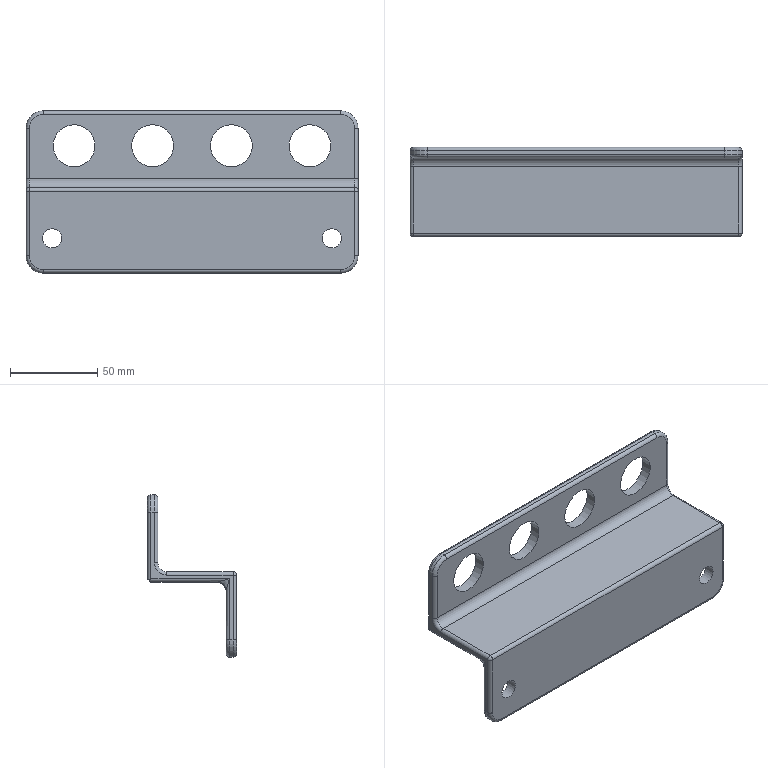Part | NX | features solid 2 | 1 solid | 54 faces | box 190 x 51 x 93 mm | volume 145209 mm3 | cylinder 29 | plane 11 | torus 10 | sphere 2 | spline 2 | commonest cylinder face diameters 4 x17 20 x4 24 x4 10 x2 11 x2
STEP:
#1=CARTESIAN_POINT('',(810.,-500.,212.));
#2=VERTEX_POINT('',#1);
#3=CARTESIAN_POINT('',(810.,-500.,200.));
#4=DIRECTION('',(0.,-1.,0.));
#5=DIRECTION('',(0.,0.,1.));
#6=AXIS2_PLACEMENT_3D('',#3,#4,#5);
#7=CIRCLE('',#6,12.);
#8=EDGE_CURVE('',#2,#2,#7,.T.);
#9=ORIENTED_EDGE('',*,*,#8,.T.);
#10=EDGE_LOOP('',(#9));
#11=FACE_BOUND('',#10,.T.);
#12=CARTESIAN_POINT('',(855.,-500.,212.));
#13=VERTEX_POINT('',#12);
#14=CARTESIAN_POINT('',(855.,-500.,200.));
#15=DIRECTION('',(0.,1.,0.));
#16=DIRECTION('',(0.,0.,1.));
#17=AXIS2_PLACEMENT_3D('',#14,#15,#16);
#18=CIRCLE('',#17,12.);
#19=EDGE_CURVE('',#13,#13,#18,.T.);
#20=ORIENTED_EDGE('',*,*,#19,.F.);
#21=EDGE_LOOP('',(#20));
#22=FACE_BOUND('',#21,.T.);
#23=CARTESIAN_POINT('',(702.5,-500.,218.));
#24=VERTEX_POINT('',#23);
#25=CARTESIAN_POINT('',(872.5,-500.,218.));
#26=VERTEX_POINT('',#25);
#27=CARTESIAN_POINT('',(877.5,-500.,218.));
#28=DIRECTION('',(-1.,0.,0.));
#29=VECTOR('',#28,1000.);
#30=LINE('',#27,#29);
#31=EDGE_CURVE('',#24,#26,#30,.F.);
#32=ORIENTED_EDGE('',*,*,#31,.T.);
#33=CARTESIAN_POINT('',(880.5,-500.,210.));
#34=VERTEX_POINT('',#33);
#35=CARTESIAN_POINT('',(872.5,-500.,210.));
#36=DIRECTION('',(0.,-1.,0.));
#37=DIRECTION('',(0.,0.,1.));
#38=AXIS2_PLACEMENT_3D('',#35,#36,#37);
#39=CIRCLE('',#38,8.);
#40=EDGE_CURVE('',#26,#34,#39,.F.);
#41=ORIENTED_EDGE('',*,*,#40,.T.);
#42=CARTESIAN_POINT('',(880.5,-500.,172.));
#43=VERTEX_POINT('',#42);
#44=CARTESIAN_POINT('',(880.5,-500.,181.));
#45=DIRECTION('',(0.,0.,1.));
#46=VECTOR('',#45,1000.);
#47=LINE('',#44,#46);
#48=EDGE_CURVE('',#34,#43,#47,.F.);
#49=ORIENTED_EDGE('',*,*,#48,.T.);
#50=CARTESIAN_POINT('',(694.5,-500.,172.));
#51=VERTEX_POINT('',#50);
#52=CARTESIAN_POINT('',(827.5,-500.,172.));
#53=DIRECTION('',(1.,0.,0.));
#54=VECTOR('',#53,1000.);
#55=LINE('',#52,#54);
#56=EDGE_CURVE('',#51,#43,#55,.T.);
#57=ORIENTED_EDGE('',*,*,#56,.F.);
#58=CARTESIAN_POINT('',(694.5,-500.,210.));
#59=VERTEX_POINT('',#58);
#60=CARTESIAN_POINT('',(694.5,-500.,181.));
#61=DIRECTION('',(0.,0.,1.));
#62=VECTOR('',#61,1000.);
#63=LINE('',#60,#62);
#64=EDGE_CURVE('',#59,#51,#63,.F.);
#65=ORIENTED_EDGE('',*,*,#64,.F.);
#66=CARTESIAN_POINT('',(702.5,-500.,210.));
#67=DIRECTION('',(0.,1.,0.));
#68=DIRECTION('',(0.,0.,1.));
#69=AXIS2_PLACEMENT_3D('',#66,#67,#68);
#70=CIRCLE('',#69,8.);
#71=EDGE_CURVE('',#24,#59,#70,.F.);
#72=ORIENTED_EDGE('',*,*,#71,.F.);
#73=EDGE_LOOP('',(#32,#41,#49,#57,#65,#72));
#74=FACE_BOUND('',#73,.T.);
#75=CARTESIAN_POINT('',(765.,-500.,212.));
#76=VERTEX_POINT('',#75);
#77=CARTESIAN_POINT('',(765.,-500.,200.));
#78=DIRECTION('',(0.,1.,0.));
#79=DIRECTION('',(0.,0.,1.));
#80=AXIS2_PLACEMENT_3D('',#77,#78,#79);
#81=CIRCLE('',#80,12.);
#82=EDGE_CURVE('',#76,#76,#81,.T.);
#83=ORIENTED_EDGE('',*,*,#82,.F.);
#84=EDGE_LOOP('',(#83));
#85=FACE_BOUND('',#84,.T.);
#86=CARTESIAN_POINT('',(720.,-500.,212.));
#87=VERTEX_POINT('',#86);
#88=CARTESIAN_POINT('',(720.,-500.,200.));
#89=DIRECTION('',(0.,-1.,0.));
#90=DIRECTION('',(0.,0.,1.));
#91=AXIS2_PLACEMENT_3D('',#88,#89,#90);
#92=CIRCLE('',#91,12.);
#93=EDGE_CURVE('',#87,#87,#92,.T.);
#94=ORIENTED_EDGE('',*,*,#93,.T.);
#95=EDGE_LOOP('',(#94));
#96=FACE_BOUND('',#95,.T.);
#97=CARTESIAN_POINT('',(767.5,-500.,170.));
#98=DIRECTION('',(0.,-1.,0.));
#99=DIRECTION('',(0.,0.,1.));
#100=AXIS2_PLACEMENT_3D('',#97,#98,#99);
#101=PLANE('',#100);
#102=ADVANCED_FACE('',(#11,#22,#74,#85,#96),#101,.F.);
#103=CARTESIAN_POINT('',(855.,-506.,212.));
#104=VERTEX_POINT('',#103);
#105=CARTESIAN_POINT('',(855.,-506.,200.));
#106=DIRECTION('',(0.,1.,0.));
#107=DIRECTION('',(0.,0.,1.));
#108=AXIS2_PLACEMENT_3D('',#105,#106,#107);
#109=CIRCLE('',#108,12.);
#110=EDGE_CURVE('',#104,#104,#109,.T.);
#111=ORIENTED_EDGE('',*,*,#110,.T.);
#112=EDGE_LOOP('',(#111));
#113=FACE_BOUND('',#112,.T.);
#114=CARTESIAN_POINT('',(810.,-506.,212.));
#115=VERTEX_POINT('',#114);
#116=CARTESIAN_POINT('',(810.,-506.,200.));
#117=DIRECTION('',(0.,-1.,0.));
#118=DIRECTION('',(0.,0.,1.));
#119=AXIS2_PLACEMENT_3D('',#116,#117,#118);
#120=CIRCLE('',#119,12.);
#121=EDGE_CURVE('',#115,#115,#120,.T.);
#122=ORIENTED_EDGE('',*,*,#121,.F.);
#123=EDGE_LOOP('',(#122));
#124=FACE_BOUND('',#123,.T.);
#125=CARTESIAN_POINT('',(694.5,-506.,181.));
#126=VERTEX_POINT('',#125);
#127=CARTESIAN_POINT('',(880.5,-506.,181.));
#128=VERTEX_POINT('',#127);
#129=CARTESIAN_POINT('',(827.5,-506.,181.));
#130=DIRECTION('',(1.,0.,0.));
#131=VECTOR('',#130,1000.);
#132=LINE('',#129,#131);
#133=EDGE_CURVE('',#126,#128,#132,.T.);
#134=ORIENTED_EDGE('',*,*,#133,.T.);
#135=CARTESIAN_POINT('',(880.5,-506.,210.));
#136=VERTEX_POINT('',#135);
#137=CARTESIAN_POINT('',(880.5,-506.,170.));
#138=DIRECTION('',(0.,0.,1.));
#139=VECTOR('',#138,1000.);
#140=LINE('',#137,#139);
#141=EDGE_CURVE('',#128,#136,#140,.T.);
#142=ORIENTED_EDGE('',*,*,#141,.T.);
#143=CARTESIAN_POINT('',(872.5,-506.,218.));
#144=VERTEX_POINT('',#143);
#145=CARTESIAN_POINT('',(872.5,-506.,210.));
#146=DIRECTION('',(0.,-1.,0.));
#147=DIRECTION('',(0.,0.,1.));
#148=AXIS2_PLACEMENT_3D('',#145,#146,#147);
#149=CIRCLE('',#148,8.);
#150=EDGE_CURVE('',#136,#144,#149,.T.);
#151=ORIENTED_EDGE('',*,*,#150,.T.);
#152=CARTESIAN_POINT('',(702.5,-506.,218.));
#153=VERTEX_POINT('',#152);
#154=CARTESIAN_POINT('',(827.5,-506.,218.));
#155=DIRECTION('',(-1.,0.,0.));
#156=VECTOR('',#155,1000.);
#157=LINE('',#154,#156);
#158=EDGE_CURVE('',#144,#153,#157,.T.);
#159=ORIENTED_EDGE('',*,*,#158,.T.);
#160=CARTESIAN_POINT('',(694.5,-506.,210.));
#161=VERTEX_POINT('',#160);
#162=CARTESIAN_POINT('',(702.5,-506.,210.));
#163=DIRECTION('',(0.,1.,0.));
#164=DIRECTION('',(0.,0.,1.));
#165=AXIS2_PLACEMENT_3D('',#162,#163,#164);
#166=CIRCLE('',#165,8.);
#167=EDGE_CURVE('',#161,#153,#166,.T.);
#168=ORIENTED_EDGE('',*,*,#167,.F.);
#169=CARTESIAN_POINT('',(694.5,-506.,170.));
#170=DIRECTION('',(0.,0.,1.));
#171=VECTOR('',#170,1000.);
#172=LINE('',#169,#171);
#173=EDGE_CURVE('',#126,#161,#172,.T.);
#174=ORIENTED_EDGE('',*,*,#173,.F.);
#175=EDGE_LOOP('',(#134,#142,#151,#159,#168,#174));
#176=FACE_BOUND('',#175,.T.);
#177=CARTESIAN_POINT('',(720.,-506.,212.));
#178=VERTEX_POINT('',#177);
#179=CARTESIAN_POINT('',(720.,-506.,200.));
#180=DIRECTION('',(0.,-1.,0.));
#181=DIRECTION('',(0.,0.,1.));
#182=AXIS2_PLACEMENT_3D('',#179,#180,#181);
#183=CIRCLE('',#182,12.);
#184=EDGE_CURVE('',#178,#178,#183,.T.);
#185=ORIENTED_EDGE('',*,*,#184,.F.);
#186=EDGE_LOOP('',(#185));
#187=FACE_BOUND('',#186,.T.);
#188=CARTESIAN_POINT('',(765.,-506.,212.));
#189=VERTEX_POINT('',#188);
#190=CARTESIAN_POINT('',(765.,-506.,200.));
#191=DIRECTION('',(0.,1.,0.));
#192=DIRECTION('',(0.,0.,1.));
#193=AXIS2_PLACEMENT_3D('',#190,#191,#192);
#194=CIRCLE('',#193,12.);
#195=EDGE_CURVE('',#189,#189,#194,.T.);
#196=ORIENTED_EDGE('',*,*,#195,.T.);
#197=EDGE_LOOP('',(#196));
#198=FACE_BOUND('',#197,.T.);
#199=CARTESIAN_POINT('',(827.5,-506.,170.));
#200=DIRECTION('',(0.,-1.,0.));
#201=DIRECTION('',(0.,0.,1.));
#202=AXIS2_PLACEMENT_3D('',#199,#200,#201);
#203=PLANE('',#202);
#204=ADVANCED_FACE('',(#113,#124,#176,#187,#198),#203,.T.);
#205=CARTESIAN_POINT('',(880.5,-502.,170.));
#206=VERTEX_POINT('',#205);
#207=CARTESIAN_POINT('',(694.5,-502.,170.));
#208=VERTEX_POINT('',#207);
#209=CARTESIAN_POINT('',(827.5,-502.,170.));
#210=DIRECTION('',(-1.,0.,0.));
#211=VECTOR('',#210,1000.);
#212=LINE('',#209,#211);
#213=EDGE_CURVE('',#206,#208,#212,.T.);
#214=ORIENTED_EDGE('',*,*,#213,.F.);
#215=CARTESIAN_POINT('',(880.5,-540.,170.));
#216=VERTEX_POINT('',#215);
#217=CARTESIAN_POINT('',(880.5,-530.,170.));
#218=DIRECTION('',(0.,-1.,0.));
#219=VECTOR('',#218,1000.);
#220=LINE('',#217,#219);
#221=EDGE_CURVE('',#216,#206,#220,.F.);
#222=ORIENTED_EDGE('',*,*,#221,.F.);
#223=CARTESIAN_POINT('',(694.5,-540.,170.));
#224=VERTEX_POINT('',#223);
#225=CARTESIAN_POINT('',(769.5,-540.,170.));
#226=DIRECTION('',(1.,0.,0.));
#227=VECTOR('',#226,1000.);
#228=LINE('',#225,#227);
#229=EDGE_CURVE('',#216,#224,#228,.F.);
#230=ORIENTED_EDGE('',*,*,#229,.T.);
#231=CARTESIAN_POINT('',(694.5,-530.,170.));
#232=DIRECTION('',(0.,-1.,0.));
#233=VECTOR('',#232,1000.);
#234=LINE('',#231,#233);
#235=EDGE_CURVE('',#224,#208,#234,.F.);
#236=ORIENTED_EDGE('',*,*,#235,.T.);
#237=EDGE_LOOP('',(#214,#222,#230,#236));
#238=FACE_BOUND('',#237,.T.);
#239=CARTESIAN_POINT('',(827.5,-530.,170.));
#240=DIRECTION('',(0.,0.,-1.));
#241=DIRECTION('',(1.,0.,0.));
#242=AXIS2_PLACEMENT_3D('',#239,#240,#241);
#243=PLANE('',#242);
#244=ADVANCED_FACE('',(#238),#243,.T.);
#245=CARTESIAN_POINT('',(694.5,-511.,176.));
#246=VERTEX_POINT('',#245);
#247=CARTESIAN_POINT('',(880.5,-511.,176.));
#248=VERTEX_POINT('',#247);
#249=CARTESIAN_POINT('',(827.5,-511.,176.));
#250=DIRECTION('',(1.,0.,0.));
#251=VECTOR('',#250,1000.);
#252=LINE('',#249,#251);
#253=EDGE_CURVE('',#246,#248,#252,.T.);
#254=ORIENTED_EDGE('',*,*,#253,.T.);
#255=CARTESIAN_POINT('',(880.5,-511.,181.));
#256=DIRECTION('',(-1.,0.,0.));
#257=DIRECTION('',(0.,0.,1.));
#258=AXIS2_PLACEMENT_3D('',#255,#256,#257);
#259=CIRCLE('',#258,5.);
#260=EDGE_CURVE('',#128,#248,#259,.T.);
#261=ORIENTED_EDGE('',*,*,#260,.F.);
#262=ORIENTED_EDGE('',*,*,#133,.F.);
#263=CARTESIAN_POINT('',(694.5,-511.,181.));
#264=DIRECTION('',(-1.,0.,0.));
#265=DIRECTION('',(0.,0.,1.));
#266=AXIS2_PLACEMENT_3D('',#263,#264,#265);
#267=CIRCLE('',#266,5.);
#268=EDGE_CURVE('',#126,#246,#267,.T.);
#269=ORIENTED_EDGE('',*,*,#268,.T.);
#270=EDGE_LOOP('',(#254,#261,#262,#269));
#271=FACE_BOUND('',#270,.T.);
#272=CARTESIAN_POINT('',(827.5,-511.,181.));
#273=DIRECTION('',(1.,0.,0.));
#274=DIRECTION('',(0.,0.,1.));
#275=AXIS2_PLACEMENT_3D('',#272,#273,#274);
#276=CYLINDRICAL_SURFACE('',#275,5.);
#277=ADVANCED_FACE('',(#271),#276,.F.);
#278=ORIENTED_EDGE('',*,*,#56,.T.);
#279=CARTESIAN_POINT('',(882.232,-501.,171.));
#280=VERTEX_POINT('',#279);
#281=CARTESIAN_POINT('',(880.5,-502.,170.));
#282=DIRECTION('',(0.,0.7071,-0.7071));
#283=DIRECTION('',(0.,0.7071,0.7071));
#284=AXIS2_PLACEMENT_3D('',#281,#282,#283);
#285=ELLIPSE('',#284,2.828,2.);
#286=EDGE_CURVE('',#43,#280,#285,.T.);
#287=ORIENTED_EDGE('',*,*,#286,.T.);
#288=CARTESIAN_POINT('',(880.5,-500.,172.));
#289=DIRECTION('',(0.,0.7071,-0.7071));
#290=DIRECTION('',(0.,-0.7071,-0.7071));
#291=AXIS2_PLACEMENT_3D('',#288,#289,#290);
#292=ELLIPSE('',#291,2.828,2.);
#293=EDGE_CURVE('',#280,#206,#292,.T.);
#294=ORIENTED_EDGE('',*,*,#293,.T.);
#295=ORIENTED_EDGE('',*,*,#213,.T.);
#296=CARTESIAN_POINT('',(692.768,-501.,171.));
#297=VERTEX_POINT('',#296);
#298=CARTESIAN_POINT('',(694.5,-500.,172.));
#299=DIRECTION('',(0.,-0.7071,0.7071));
#300=DIRECTION('',(0.,-0.7071,-0.7071));
#301=AXIS2_PLACEMENT_3D('',#298,#299,#300);
#302=ELLIPSE('',#301,2.828,2.);
#303=EDGE_CURVE('',#297,#208,#302,.T.);
#304=ORIENTED_EDGE('',*,*,#303,.F.);
#305=CARTESIAN_POINT('',(694.5,-502.,170.));
#306=DIRECTION('',(0.,-0.7071,0.7071));
#307=DIRECTION('',(0.,0.7071,0.7071));
#308=AXIS2_PLACEMENT_3D('',#305,#306,#307);
#309=ELLIPSE('',#308,2.828,2.);
#310=EDGE_CURVE('',#51,#297,#309,.T.);
#311=ORIENTED_EDGE('',*,*,#310,.F.);
#312=EDGE_LOOP('',(#278,#287,#294,#295,#304,#311));
#313=FACE_BOUND('',#312,.T.);
#314=CARTESIAN_POINT('',(827.5,-500.,172.));
#315=DIRECTION('',(0.,-0.7071,0.7071));
#316=DIRECTION('',(0.,-0.7071,-0.7071));
#317=AXIS2_PLACEMENT_3D('',#314,#315,#316);
#318=PLANE('',#317);
#319=ADVANCED_FACE('',(#313),#318,.F.);
#320=CARTESIAN_POINT('',(694.5,-549.,176.));
#321=VERTEX_POINT('',#320);
#322=CARTESIAN_POINT('',(880.5,-549.,176.));
#323=VERTEX_POINT('',#322);
#324=CARTESIAN_POINT('',(769.5,-549.,176.));
#325=DIRECTION('',(1.,0.,0.));
#326=VECTOR('',#325,1000.);
#327=LINE('',#324,#326);
#328=EDGE_CURVE('',#321,#323,#327,.T.);
#329=ORIENTED_EDGE('',*,*,#328,.T.);
#330=CARTESIAN_POINT('',(880.5,-551.,176.));
#331=DIRECTION('',(0.,-1.,0.));
#332=VECTOR('',#331,1000.);
#333=LINE('',#330,#332);
#334=EDGE_CURVE('',#323,#248,#333,.F.);
#335=ORIENTED_EDGE('',*,*,#334,.T.);
#336=ORIENTED_EDGE('',*,*,#253,.F.);
#337=CARTESIAN_POINT('',(694.5,-551.,176.));
#338=DIRECTION('',(0.,-1.,0.));
#339=VECTOR('',#338,1000.);
#340=LINE('',#337,#339);
#341=EDGE_CURVE('',#321,#246,#340,.F.);
#342=ORIENTED_EDGE('',*,*,#341,.F.);
#343=EDGE_LOOP('',(#329,#335,#336,#342));
#344=FACE_BOUND('',#343,.T.);
#345=CARTESIAN_POINT('',(769.5,-551.,176.));
#346=DIRECTION('',(0.,0.,1.));
#347=DIRECTION('',(1.,0.,0.));
#348=AXIS2_PLACEMENT_3D('',#345,#346,#347);
#349=PLANE('',#348);
#350=ADVANCED_FACE('',(#344),#349,.T.);
#351=CARTESIAN_POINT('',(873.,-551.,147.));
#352=VERTEX_POINT('',#351);
#353=CARTESIAN_POINT('',(867.5,-551.,147.));
#354=DIRECTION('',(0.,-1.,0.));
#355=DIRECTION('',(1.,0.,0.));
#356=AXIS2_PLACEMENT_3D('',#353,#354,#355);
#357=CIRCLE('',#356,5.5);
#358=EDGE_CURVE('',#352,#352,#357,.T.);
#359=ORIENTED_EDGE('',*,*,#358,.F.);
#360=EDGE_LOOP('',(#359));
#361=FACE_BOUND('',#360,.T.);
#362=CARTESIAN_POINT('',(872.5,-551.,129.));
#363=VERTEX_POINT('',#362);
#364=CARTESIAN_POINT('',(702.5,-551.,129.));
#365=VERTEX_POINT('',#364);
#366=CARTESIAN_POINT('',(827.5,-551.,129.));
#367=DIRECTION('',(1.,0.,0.));
#368=VECTOR('',#367,1000.);
#369=LINE('',#366,#368);
#370=EDGE_CURVE('',#363,#365,#369,.F.);
#371=ORIENTED_EDGE('',*,*,#370,.F.);
#372=CARTESIAN_POINT('',(880.5,-551.,137.));
#373=VERTEX_POINT('',#372);
#374=CARTESIAN_POINT('',(872.5,-551.,137.));
#375=DIRECTION('',(0.,1.,0.));
#376=DIRECTION('',(-1.,0.,0.));
#377=AXIS2_PLACEMENT_3D('',#374,#375,#376);
#378=CIRCLE('',#377,8.);
#379=EDGE_CURVE('',#373,#363,#378,.T.);
#380=ORIENTED_EDGE('',*,*,#379,.F.);
#381=CARTESIAN_POINT('',(880.5,-551.,174.));
#382=VERTEX_POINT('',#381);
#383=CARTESIAN_POINT('',(880.5,-551.,176.));
#384=DIRECTION('',(0.,0.,1.));
#385=VECTOR('',#384,1000.);
#386=LINE('',#383,#385);
#387=EDGE_CURVE('',#373,#382,#386,.T.);
#388=ORIENTED_EDGE('',*,*,#387,.T.);
#389=CARTESIAN_POINT('',(694.5,-551.,174.));
#390=VERTEX_POINT('',#389);
#391=CARTESIAN_POINT('',(769.5,-551.,174.));
#392=DIRECTION('',(-1.,0.,0.));
#393=VECTOR('',#392,1000.);
#394=LINE('',#391,#393);
#395=EDGE_CURVE('',#382,#390,#394,.T.);
#396=ORIENTED_EDGE('',*,*,#395,.T.);
#397=CARTESIAN_POINT('',(694.5,-551.,137.));
#398=VERTEX_POINT('',#397);
#399=CARTESIAN_POINT('',(694.5,-551.,176.));
#400=DIRECTION('',(0.,0.,1.));
#401=VECTOR('',#400,1000.);
#402=LINE('',#399,#401);
#403=EDGE_CURVE('',#398,#390,#402,.T.);
#404=ORIENTED_EDGE('',*,*,#403,.F.);
#405=CARTESIAN_POINT('',(702.5,-551.,137.));
#406=DIRECTION('',(0.,-1.,0.));
#407=DIRECTION('',(1.,0.,0.));
#408=AXIS2_PLACEMENT_3D('',#405,#406,#407);
#409=CIRCLE('',#408,8.);
#410=EDGE_CURVE('',#398,#365,#409,.T.);
#411=ORIENTED_EDGE('',*,*,#410,.T.);
#412=EDGE_LOOP('',(#371,#380,#388,#396,#404,#411));
#413=FACE_BOUND('',#412,.T.);
#414=CARTESIAN_POINT('',(702.,-551.,147.));
#415=VERTEX_POINT('',#414);
#416=CARTESIAN_POINT('',(707.5,-551.,147.));
#417=DIRECTION('',(0.,1.,0.));
#418=DIRECTION('',(-1.,0.,0.));
#419=AXIS2_PLACEMENT_3D('',#416,#417,#418);
#420=CIRCLE('',#419,5.5);
#421=EDGE_CURVE('',#415,#415,#420,.T.);
#422=ORIENTED_EDGE('',*,*,#421,.T.);
#423=EDGE_LOOP('',(#422));
#424=FACE_BOUND('',#423,.T.);
#425=CARTESIAN_POINT('',(769.5,-551.,176.));
#426=DIRECTION('',(0.,1.,0.));
#427=DIRECTION('',(0.,0.,-1.));
#428=AXIS2_PLACEMENT_3D('',#425,#426,#427);
#429=PLANE('',#428);
#430=ADVANCED_FACE('',(#361,#413,#424),#429,.F.);
#431=ORIENTED_EDGE('',*,*,#395,.F.);
#432=CARTESIAN_POINT('',(880.5,-549.,174.));
#433=DIRECTION('',(-1.,0.,0.));
#434=DIRECTION('',(0.,1.,0.));
#435=AXIS2_PLACEMENT_3D('',#432,#433,#434);
#436=CIRCLE('',#435,2.);
#437=EDGE_CURVE('',#382,#323,#436,.T.);
#438=ORIENTED_EDGE('',*,*,#437,.T.);
#439=ORIENTED_EDGE('',*,*,#328,.F.);
#440=CARTESIAN_POINT('',(694.5,-549.,174.));
#441=DIRECTION('',(-1.,0.,0.));
#442=DIRECTION('',(0.,1.,0.));
#443=AXIS2_PLACEMENT_3D('',#440,#441,#442);
#444=CIRCLE('',#443,2.);
#445=EDGE_CURVE('',#390,#321,#444,.T.);
#446=ORIENTED_EDGE('',*,*,#445,.F.);
#447=EDGE_LOOP('',(#431,#438,#439,#446));
#448=FACE_BOUND('',#447,.T.);
#449=CARTESIAN_POINT('',(769.5,-549.,174.));
#450=DIRECTION('',(-1.,0.,0.));
#451=DIRECTION('',(0.,1.,0.));
#452=AXIS2_PLACEMENT_3D('',#449,#450,#451);
#453=CYLINDRICAL_SURFACE('',#452,2.);
#454=ADVANCED_FACE('',(#448),#453,.T.);
#455=CARTESIAN_POINT('',(873.,-545.,147.));
#456=VERTEX_POINT('',#455);
#457=CARTESIAN_POINT('',(867.5,-545.,147.));
#458=DIRECTION('',(0.,-1.,0.));
#459=DIRECTION('',(1.,0.,0.));
#460=AXIS2_PLACEMENT_3D('',#457,#458,#459);
#461=CIRCLE('',#460,5.5);
#462=EDGE_CURVE('',#456,#456,#461,.T.);
#463=ORIENTED_EDGE('',*,*,#462,.T.);
#464=EDGE_LOOP('',(#463));
#465=FACE_BOUND('',#464,.T.);
#466=CARTESIAN_POINT('',(694.5,-545.,165.));
#467=VERTEX_POINT('',#466);
#468=CARTESIAN_POINT('',(880.5,-545.,165.));
#469=VERTEX_POINT('',#468);
#470=CARTESIAN_POINT('',(885.5,-545.,165.));
#471=DIRECTION('',(1.,0.,0.));
#472=VECTOR('',#471,1000.);
#473=LINE('',#470,#472);
#474=EDGE_CURVE('',#467,#469,#473,.T.);
#475=ORIENTED_EDGE('',*,*,#474,.T.);
#476=CARTESIAN_POINT('',(880.5,-545.,137.));
#477=VERTEX_POINT('',#476);
#478=CARTESIAN_POINT('',(880.5,-545.,157.));
#479=DIRECTION('',(0.,0.,-1.));
#480=VECTOR('',#479,1000.);
#481=LINE('',#478,#480);
#482=EDGE_CURVE('',#477,#469,#481,.F.);
#483=ORIENTED_EDGE('',*,*,#482,.F.);
#484=CARTESIAN_POINT('',(872.5,-545.,129.));
#485=VERTEX_POINT('',#484);
#486=CARTESIAN_POINT('',(872.5,-545.,137.));
#487=DIRECTION('',(0.,-1.,0.));
#488=DIRECTION('',(1.,0.,0.));
#489=AXIS2_PLACEMENT_3D('',#486,#487,#488);
#490=CIRCLE('',#489,8.);
#491=EDGE_CURVE('',#485,#477,#490,.T.);
#492=ORIENTED_EDGE('',*,*,#491,.F.);
#493=CARTESIAN_POINT('',(702.5,-545.,129.));
#494=VERTEX_POINT('',#493);
#495=CARTESIAN_POINT('',(827.5,-545.,129.));
#496=DIRECTION('',(-1.,0.,0.));
#497=VECTOR('',#496,1000.);
#498=LINE('',#495,#497);
#499=EDGE_CURVE('',#494,#485,#498,.F.);
#500=ORIENTED_EDGE('',*,*,#499,.F.);
#501=CARTESIAN_POINT('',(694.5,-545.,137.));
#502=VERTEX_POINT('',#501);
#503=CARTESIAN_POINT('',(702.5,-545.,137.));
#504=DIRECTION('',(0.,1.,0.));
#505=DIRECTION('',(-1.,0.,0.));
#506=AXIS2_PLACEMENT_3D('',#503,#504,#505);
#507=CIRCLE('',#506,8.);
#508=EDGE_CURVE('',#494,#502,#507,.T.);
#509=ORIENTED_EDGE('',*,*,#508,.T.);
#510=CARTESIAN_POINT('',(694.5,-545.,157.));
#511=DIRECTION('',(0.,0.,-1.));
#512=VECTOR('',#511,1000.);
#513=LINE('',#510,#512);
#514=EDGE_CURVE('',#502,#467,#513,.F.);
#515=ORIENTED_EDGE('',*,*,#514,.T.);
#516=EDGE_LOOP('',(#475,#483,#492,#500,#509,#515));
#517=FACE_BOUND('',#516,.T.);
#518=CARTESIAN_POINT('',(702.,-545.,147.));
#519=VERTEX_POINT('',#518);
#520=CARTESIAN_POINT('',(707.5,-545.,147.));
#521=DIRECTION('',(0.,1.,0.));
#522=DIRECTION('',(-1.,0.,0.));
#523=AXIS2_PLACEMENT_3D('',#520,#521,#522);
#524=CIRCLE('',#523,5.5);
#525=EDGE_CURVE('',#519,#519,#524,.T.);
#526=ORIENTED_EDGE('',*,*,#525,.F.);
#527=EDGE_LOOP('',(#526));
#528=FACE_BOUND('',#527,.T.);
#529=CARTESIAN_POINT('',(827.5,-545.,157.));
#530=DIRECTION('',(0.,1.,0.));
#531=DIRECTION('',(1.,0.,0.));
#532=AXIS2_PLACEMENT_3D('',#529,#530,#531);
#533=PLANE('',#532);
#534=ADVANCED_FACE('',(#465,#517,#528),#533,.T.);
#535=ORIENTED_EDGE('',*,*,#229,.F.);
#536=CARTESIAN_POINT('',(880.5,-540.,165.));
#537=DIRECTION('',(1.,0.,0.));
#538=DIRECTION('',(0.,-1.,0.));
#539=AXIS2_PLACEMENT_3D('',#536,#537,#538);
#540=CIRCLE('',#539,5.);
#541=EDGE_CURVE('',#216,#469,#540,.T.);
#542=ORIENTED_EDGE('',*,*,#541,.T.);
#543=ORIENTED_EDGE('',*,*,#474,.F.);
#544=CARTESIAN_POINT('',(694.5,-540.,165.));
#545=DIRECTION('',(1.,0.,0.));
#546=DIRECTION('',(0.,-1.,0.));
#547=AXIS2_PLACEMENT_3D('',#544,#545,#546);
#548=CIRCLE('',#547,5.);
#549=EDGE_CURVE('',#224,#467,#548,.T.);
#550=ORIENTED_EDGE('',*,*,#549,.F.);
#551=EDGE_LOOP('',(#535,#542,#543,#550));
#552=FACE_BOUND('',#551,.T.);
#553=CARTESIAN_POINT('',(827.5,-540.,165.));
#554=DIRECTION('',(-1.,0.,0.));
#555=DIRECTION('',(0.,1.,0.));
#556=AXIS2_PLACEMENT_3D('',#553,#554,#555);
#557=CYLINDRICAL_SURFACE('',#556,5.);
#558=ADVANCED_FACE('',(#552),#557,.F.);
#559=CARTESIAN_POINT('',(702.5,-504.,220.));
#560=VERTEX_POINT('',#559);
#561=CARTESIAN_POINT('',(872.5,-504.,220.));
#562=VERTEX_POINT('',#561);
#563=CARTESIAN_POINT('',(767.5,-504.,220.));
#564=DIRECTION('',(1.,0.,0.));
#565=VECTOR('',#564,1000.);
#566=LINE('',#563,#565);
#567=EDGE_CURVE('',#560,#562,#566,.T.);
#568=ORIENTED_EDGE('',*,*,#567,.T.);
#569=CARTESIAN_POINT('',(872.5,-502.,220.));
#570=VERTEX_POINT('',#569);
#571=CARTESIAN_POINT('',(872.5,-506.,220.));
#572=DIRECTION('',(0.,-1.,0.));
#573=VECTOR('',#572,1000.);
#574=LINE('',#571,#573);
#575=EDGE_CURVE('',#562,#570,#574,.F.);
#576=ORIENTED_EDGE('',*,*,#575,.T.);
#577=CARTESIAN_POINT('',(702.5,-502.,220.));
#578=VERTEX_POINT('',#577);
#579=CARTESIAN_POINT('',(777.5,-502.,220.));
#580=DIRECTION('',(1.,0.,0.));
#581=VECTOR('',#580,1000.);
#582=LINE('',#579,#581);
#583=EDGE_CURVE('',#570,#578,#582,.F.);
#584=ORIENTED_EDGE('',*,*,#583,.T.);
#585=CARTESIAN_POINT('',(702.5,-506.,220.));
#586=DIRECTION('',(0.,-1.,0.));
#587=VECTOR('',#586,1000.);
#588=LINE('',#585,#587);
#589=EDGE_CURVE('',#560,#578,#588,.F.);
#590=ORIENTED_EDGE('',*,*,#589,.F.);
#591=EDGE_LOOP('',(#568,#576,#584,#590));
#592=FACE_BOUND('',#591,.T.);
#593=CARTESIAN_POINT('',(767.5,-506.,220.));
#594=DIRECTION('',(0.,0.,-1.));
#595=DIRECTION('',(1.,0.,0.));
#596=AXIS2_PLACEMENT_3D('',#593,#594,#595);
#597=PLANE('',#596);
#598=ADVANCED_FACE('',(#592),#597,.F.);
#599=ORIENTED_EDGE('',*,*,#575,.F.);
#600=CARTESIAN_POINT('',(882.5,-504.,210.));
#601=VERTEX_POINT('',#600);
#602=CARTESIAN_POINT('',(872.5,-504.,210.));
#603=DIRECTION('',(0.,-1.,0.));
#604=DIRECTION('',(0.,0.,1.));
#605=AXIS2_PLACEMENT_3D('',#602,#603,#604);
#606=CIRCLE('',#605,10.);
#607=EDGE_CURVE('',#562,#601,#606,.F.);
#608=ORIENTED_EDGE('',*,*,#607,.T.);
#609=CARTESIAN_POINT('',(882.5,-502.,210.));
#610=VERTEX_POINT('',#609);
#611=CARTESIAN_POINT('',(882.5,-476.,210.));
#612=DIRECTION('',(0.,1.,0.));
#613=VECTOR('',#612,1000.);
#614=LINE('',#611,#613);
#615=EDGE_CURVE('',#610,#601,#614,.F.);
#616=ORIENTED_EDGE('',*,*,#615,.F.);
#617=CARTESIAN_POINT('',(872.5,-502.,210.));
#618=DIRECTION('',(0.,-1.,0.));
#619=DIRECTION('',(0.,0.,1.));
#620=AXIS2_PLACEMENT_3D('',#617,#618,#619);
#621=CIRCLE('',#620,10.);
#622=EDGE_CURVE('',#610,#570,#621,.T.);
#623=ORIENTED_EDGE('',*,*,#622,.T.);
#624=EDGE_LOOP('',(#599,#608,#616,#623));
#625=FACE_BOUND('',#624,.T.);
#626=CARTESIAN_POINT('',(872.5,-476.,210.));
#627=DIRECTION('',(0.,1.,0.));
#628=DIRECTION('',(0.,0.,-1.));
#629=AXIS2_PLACEMENT_3D('',#626,#627,#628);
#630=CYLINDRICAL_SURFACE('',#629,10.);
#631=ADVANCED_FACE('',(#625),#630,.T.);
#632=ORIENTED_EDGE('',*,*,#158,.F.);
#633=CARTESIAN_POINT('',(872.5,-504.,218.));
#634=DIRECTION('',(1.,0.,0.));
#635=DIRECTION('',(0.,0.,1.));
#636=AXIS2_PLACEMENT_3D('',#633,#634,#635);
#637=CIRCLE('',#636,2.);
#638=EDGE_CURVE('',#562,#144,#637,.T.);
#639=ORIENTED_EDGE('',*,*,#638,.F.);
#640=ORIENTED_EDGE('',*,*,#567,.F.);
#641=CARTESIAN_POINT('',(702.5,-504.,218.));
#642=DIRECTION('',(1.,0.,0.));
#643=DIRECTION('',(0.,0.,1.));
#644=AXIS2_PLACEMENT_3D('',#641,#642,#643);
#645=CIRCLE('',#644,2.);
#646=EDGE_CURVE('',#560,#153,#645,.T.);
#647=ORIENTED_EDGE('',*,*,#646,.T.);
#648=EDGE_LOOP('',(#632,#639,#640,#647));
#649=FACE_BOUND('',#648,.T.);
#650=CARTESIAN_POINT('',(767.5,-504.,218.));
#651=DIRECTION('',(-1.,0.,0.));
#652=DIRECTION('',(0.,0.,-1.));
#653=AXIS2_PLACEMENT_3D('',#650,#651,#652);
#654=CYLINDRICAL_SURFACE('',#653,2.);
#655=ADVANCED_FACE('',(#649),#654,.T.);
#656=ORIENTED_EDGE('',*,*,#583,.F.);
#657=CARTESIAN_POINT('',(872.5,-502.,218.));
#658=DIRECTION('',(1.,0.,0.));
#659=DIRECTION('',(0.,0.,1.));
#660=AXIS2_PLACEMENT_3D('',#657,#658,#659);
#661=CIRCLE('',#660,2.);
#662=EDGE_CURVE('',#26,#570,#661,.T.);
#663=ORIENTED_EDGE('',*,*,#662,.F.);
#664=ORIENTED_EDGE('',*,*,#31,.F.);
#665=CARTESIAN_POINT('',(702.5,-502.,218.));
#666=DIRECTION('',(1.,0.,0.));
#667=DIRECTION('',(0.,0.,1.));
#668=AXIS2_PLACEMENT_3D('',#665,#666,#667);
#669=CIRCLE('',#668,2.);
#670=EDGE_CURVE('',#24,#578,#669,.T.);
#671=ORIENTED_EDGE('',*,*,#670,.T.);
#672=EDGE_LOOP('',(#656,#663,#664,#671));
#673=FACE_BOUND('',#672,.T.);
#674=CARTESIAN_POINT('',(767.5,-502.,218.));
#675=DIRECTION('',(1.,0.,0.));
#676=DIRECTION('',(0.,0.,1.));
#677=AXIS2_PLACEMENT_3D('',#674,#675,#676);
#678=CYLINDRICAL_SURFACE('',#677,2.);
#679=ADVANCED_FACE('',(#673),#678,.T.);
#680=ORIENTED_EDGE('',*,*,#121,.T.);
#681=EDGE_LOOP('',(#680));
#682=FACE_BOUND('',#681,.T.);
#683=ORIENTED_EDGE('',*,*,#8,.F.);
#684=EDGE_LOOP('',(#683));
#685=FACE_BOUND('',#684,.T.);
#686=CARTESIAN_POINT('',(810.,-500.,200.));
#687=DIRECTION('',(0.,-1.,0.));
#688=DIRECTION('',(0.,0.,1.));
#689=AXIS2_PLACEMENT_3D('',#686,#687,#688);
#690=CYLINDRICAL_SURFACE('',#689,12.);
#691=ADVANCED_FACE('',(#682,#685),#690,.F.);
#692=ORIENTED_EDGE('',*,*,#110,.F.);
#693=EDGE_LOOP('',(#692));
#694=FACE_BOUND('',#693,.T.);
#695=ORIENTED_EDGE('',*,*,#19,.T.);
#696=EDGE_LOOP('',(#695));
#697=FACE_BOUND('',#696,.T.);
#698=CARTESIAN_POINT('',(855.,-500.,200.));
#699=DIRECTION('',(0.,-1.,0.));
#700=DIRECTION('',(0.,0.,1.));
#701=AXIS2_PLACEMENT_3D('',#698,#699,#700);
#702=CYLINDRICAL_SURFACE('',#701,12.);
#703=ADVANCED_FACE('',(#694,#697),#702,.F.);
#704=ORIENTED_EDGE('',*,*,#638,.T.);
#705=ORIENTED_EDGE('',*,*,#150,.F.);
#706=CARTESIAN_POINT('',(880.5,-504.,210.));
#707=DIRECTION('',(0.,0.,-1.));
#708=DIRECTION('',(1.,0.,0.));
#709=AXIS2_PLACEMENT_3D('',#706,#707,#708);
#710=CIRCLE('',#709,2.);
#711=EDGE_CURVE('',#601,#136,#710,.T.);
#712=ORIENTED_EDGE('',*,*,#711,.F.);
#713=ORIENTED_EDGE('',*,*,#607,.F.);
#714=EDGE_LOOP('',(#704,#705,#712,#713));
#715=FACE_BOUND('',#714,.T.);
#716=CARTESIAN_POINT('',(872.5,-504.,210.));
#717=DIRECTION('',(0.,-1.,0.));
#718=DIRECTION('',(0.,0.,1.));
#719=AXIS2_PLACEMENT_3D('',#716,#717,#718);
#720=TOROIDAL_SURFACE('',#719,8.,2.);
#721=ADVANCED_FACE('',(#715),#720,.T.);
#722=ORIENTED_EDGE('',*,*,#662,.T.);
#723=ORIENTED_EDGE('',*,*,#622,.F.);
#724=CARTESIAN_POINT('',(880.5,-502.,210.));
#725=DIRECTION('',(0.,0.,1.));
#726=DIRECTION('',(-1.,0.,0.));
#727=AXIS2_PLACEMENT_3D('',#724,#725,#726);
#728=CIRCLE('',#727,2.);
#729=EDGE_CURVE('',#610,#34,#728,.T.);
#730=ORIENTED_EDGE('',*,*,#729,.T.);
#731=ORIENTED_EDGE('',*,*,#40,.F.);
#732=EDGE_LOOP('',(#722,#723,#730,#731));
#733=FACE_BOUND('',#732,.T.);
#734=CARTESIAN_POINT('',(872.5,-502.,210.));
#735=DIRECTION('',(0.,-1.,0.));
#736=DIRECTION('',(0.,0.,1.));
#737=AXIS2_PLACEMENT_3D('',#734,#735,#736);
#738=TOROIDAL_SURFACE('',#737,8.,2.);
#739=ADVANCED_FACE('',(#733),#738,.T.);
#740=ORIENTED_EDGE('',*,*,#141,.F.);
#741=CARTESIAN_POINT('',(882.5,-504.,181.));
#742=VERTEX_POINT('',#741);
#743=CARTESIAN_POINT('',(880.5,-504.,181.));
#744=DIRECTION('',(0.,0.,-1.));
#745=DIRECTION('',(1.,0.,0.));
#746=AXIS2_PLACEMENT_3D('',#743,#744,#745);
#747=CIRCLE('',#746,2.);
#748=EDGE_CURVE('',#128,#742,#747,.F.);
#749=ORIENTED_EDGE('',*,*,#748,.T.);
#750=CARTESIAN_POINT('',(882.5,-504.,170.));
#751=DIRECTION('',(0.,0.,1.));
#752=VECTOR('',#751,1000.);
#753=LINE('',#750,#752);
#754=EDGE_CURVE('',#601,#742,#753,.F.);
#755=ORIENTED_EDGE('',*,*,#754,.F.);
#756=ORIENTED_EDGE('',*,*,#711,.T.);
#757=EDGE_LOOP('',(#740,#749,#755,#756));
#758=FACE_BOUND('',#757,.T.);
#759=CARTESIAN_POINT('',(880.5,-504.,170.));
#760=DIRECTION('',(0.,0.,1.));
#761=DIRECTION('',(-1.,0.,0.));
#762=AXIS2_PLACEMENT_3D('',#759,#760,#761);
#763=CYLINDRICAL_SURFACE('',#762,2.);
#764=ADVANCED_FACE('',(#758),#763,.T.);
#765=CARTESIAN_POINT('',(882.5,-502.,172.));
#766=VERTEX_POINT('',#765);
#767=CARTESIAN_POINT('',(882.5,-502.,220.));
#768=DIRECTION('',(0.,0.,1.));
#769=VECTOR('',#768,1000.);
#770=LINE('',#767,#769);
#771=EDGE_CURVE('',#766,#610,#770,.T.);
#772=ORIENTED_EDGE('',*,*,#771,.F.);
#773=CARTESIAN_POINT('',(880.5,-502.,172.));
#774=DIRECTION('',(0.,-0.7071,-0.7071));
#775=DIRECTION('',(0.,-0.7071,0.7071));
#776=AXIS2_PLACEMENT_3D('',#773,#774,#775);
#777=ELLIPSE('',#776,2.828,2.);
#778=EDGE_CURVE('',#766,#280,#777,.F.);
#779=ORIENTED_EDGE('',*,*,#778,.T.);
#780=ORIENTED_EDGE('',*,*,#286,.F.);
#781=ORIENTED_EDGE('',*,*,#48,.F.);
#782=ORIENTED_EDGE('',*,*,#729,.F.);
#783=EDGE_LOOP('',(#772,#779,#780,#781,#782));
#784=FACE_BOUND('',#783,.T.);
#785=CARTESIAN_POINT('',(880.5,-502.,170.));
#786=DIRECTION('',(0.,0.,-1.));
#787=DIRECTION('',(1.,0.,0.));
#788=AXIS2_PLACEMENT_3D('',#785,#786,#787);
#789=CYLINDRICAL_SURFACE('',#788,2.);
#790=ADVANCED_FACE('',(#784),#789,.T.);
#791=CARTESIAN_POINT('',(882.5,-547.,172.));
#792=VERTEX_POINT('',#791);
#793=CARTESIAN_POINT('',(882.5,-547.,137.));
#794=VERTEX_POINT('',#793);
#795=CARTESIAN_POINT('',(882.5,-547.,157.));
#796=DIRECTION('',(0.,0.,-1.));
#797=VECTOR('',#796,1000.);
#798=LINE('',#795,#797);
#799=EDGE_CURVE('',#792,#794,#798,.T.);
#800=ORIENTED_EDGE('',*,*,#799,.F.);
#801=CARTESIAN_POINT('',(882.5,-530.,172.));
#802=DIRECTION('',(0.,-1.,0.));
#803=VECTOR('',#802,1000.);
#804=LINE('',#801,#803);
#805=EDGE_CURVE('',#766,#792,#804,.T.);
#806=ORIENTED_EDGE('',*,*,#805,.F.);
#807=ORIENTED_EDGE('',*,*,#771,.T.);
#808=ORIENTED_EDGE('',*,*,#615,.T.);
#809=ORIENTED_EDGE('',*,*,#754,.T.);
#810=CARTESIAN_POINT('',(882.5,-511.,174.));
#811=VERTEX_POINT('',#810);
#812=CARTESIAN_POINT('',(882.5,-511.,181.));
#813=DIRECTION('',(-1.,0.,0.));
#814=DIRECTION('',(0.,0.,1.));
#815=AXIS2_PLACEMENT_3D('',#812,#813,#814);
#816=CIRCLE('',#815,7.);
#817=EDGE_CURVE('',#811,#742,#816,.F.);
#818=ORIENTED_EDGE('',*,*,#817,.F.);
#819=CARTESIAN_POINT('',(882.5,-549.,174.));
#820=VERTEX_POINT('',#819);
#821=CARTESIAN_POINT('',(882.5,-476.,174.));
#822=DIRECTION('',(0.,-1.,0.));
#823=VECTOR('',#822,1000.);
#824=LINE('',#821,#823);
#825=EDGE_CURVE('',#811,#820,#824,.T.);
#826=ORIENTED_EDGE('',*,*,#825,.T.);
#827=CARTESIAN_POINT('',(882.5,-549.,137.));
#828=VERTEX_POINT('',#827);
#829=CARTESIAN_POINT('',(882.5,-549.,170.));
#830=DIRECTION('',(0.,0.,-1.));
#831=VECTOR('',#830,1000.);
#832=LINE('',#829,#831);
#833=EDGE_CURVE('',#820,#828,#832,.T.);
#834=ORIENTED_EDGE('',*,*,#833,.T.);
#835=CARTESIAN_POINT('',(882.5,-545.,137.));
#836=DIRECTION('',(0.,-1.,0.));
#837=VECTOR('',#836,1000.);
#838=LINE('',#835,#837);
#839=EDGE_CURVE('',#794,#828,#838,.T.);
#840=ORIENTED_EDGE('',*,*,#839,.F.);
#841=EDGE_LOOP('',(#800,#806,#807,#808,#809,#818,#826,#834,#840));
#842=FACE_BOUND('',#841,.T.);
#843=CARTESIAN_POINT('',(882.5,-476.,170.));
#844=DIRECTION('',(1.,0.,0.));
#845=DIRECTION('',(0.,0.,1.));
#846=AXIS2_PLACEMENT_3D('',#843,#844,#845);
#847=PLANE('',#846);
#848=ADVANCED_FACE('',(#842),#847,.T.);
#849=ORIENTED_EDGE('',*,*,#805,.T.);
#850=CARTESIAN_POINT('',(880.5,-547.,172.));
#851=DIRECTION('',(0.,0.2747,0.9615));
#852=DIRECTION('',(0.,0.9615,-0.2747));
#853=AXIS2_PLACEMENT_3D('',#850,#851,#852);
#854=ELLIPSE('',#853,7.28,2.);
#855=EDGE_CURVE('',#792,#216,#854,.T.);
#856=ORIENTED_EDGE('',*,*,#855,.T.);
#857=ORIENTED_EDGE('',*,*,#221,.T.);
#858=ORIENTED_EDGE('',*,*,#293,.F.);
#859=ORIENTED_EDGE('',*,*,#778,.F.);
#860=EDGE_LOOP('',(#849,#856,#857,#858,#859));
#861=FACE_BOUND('',#860,.T.);
#862=CARTESIAN_POINT('',(880.5,-530.,172.));
#863=DIRECTION('',(0.,-1.,0.));
#864=DIRECTION('',(0.,0.,-1.));
#865=AXIS2_PLACEMENT_3D('',#862,#863,#864);
#866=CYLINDRICAL_SURFACE('',#865,2.);
#867=ADVANCED_FACE('',(#861),#866,.T.);
#868=CARTESIAN_POINT('',(880.5,-511.,174.));
#869=DIRECTION('',(0.,-1.,0.));
#870=DIRECTION('',(0.,0.,1.));
#871=AXIS2_PLACEMENT_3D('',#868,#869,#870);
#872=CIRCLE('',#871,2.);
#873=EDGE_CURVE('',#811,#248,#872,.T.);
#874=ORIENTED_EDGE('',*,*,#873,.F.);
#875=ORIENTED_EDGE('',*,*,#817,.T.);
#876=ORIENTED_EDGE('',*,*,#748,.F.);
#877=ORIENTED_EDGE('',*,*,#260,.T.);
#878=EDGE_LOOP('',(#874,#875,#876,#877));
#879=FACE_BOUND('',#878,.T.);
#880=CARTESIAN_POINT('',(880.5,-511.,181.));
#881=DIRECTION('',(1.,0.,0.));
#882=DIRECTION('',(0.,0.,1.));
#883=AXIS2_PLACEMENT_3D('',#880,#881,#882);
#884=TOROIDAL_SURFACE('',#883,7.,2.);
#885=ADVANCED_FACE('',(#879),#884,.T.);
#886=CARTESIAN_POINT('',(880.5,-549.,174.));
#887=DIRECTION('',(0.,1.,0.));
#888=DIRECTION('',(1.,0.,0.));
#889=AXIS2_PLACEMENT_3D('',#886,#887,#888);
#890=CIRCLE('',#889,2.);
#891=EDGE_CURVE('',#323,#820,#890,.T.);
#892=ORIENTED_EDGE('',*,*,#891,.T.);
#893=ORIENTED_EDGE('',*,*,#825,.F.);
#894=ORIENTED_EDGE('',*,*,#873,.T.);
#895=ORIENTED_EDGE('',*,*,#334,.F.);
#896=EDGE_LOOP('',(#892,#893,#894,#895));
#897=FACE_BOUND('',#896,.T.);
#898=CARTESIAN_POINT('',(880.5,-551.,174.));
#899=DIRECTION('',(0.,1.,0.));
#900=DIRECTION('',(1.,0.,0.));
#901=AXIS2_PLACEMENT_3D('',#898,#899,#900);
#902=CYLINDRICAL_SURFACE('',#901,2.);
#903=ADVANCED_FACE('',(#897),#902,.T.);
#904=ORIENTED_EDGE('',*,*,#387,.F.);
#905=CARTESIAN_POINT('',(880.5,-549.,137.));
#906=DIRECTION('',(0.,0.,-1.));
#907=DIRECTION('',(0.,-1.,0.));
#908=AXIS2_PLACEMENT_3D('',#905,#906,#907);
#909=CIRCLE('',#908,2.);
#910=EDGE_CURVE('',#828,#373,#909,.T.);
#911=ORIENTED_EDGE('',*,*,#910,.F.);
#912=ORIENTED_EDGE('',*,*,#833,.F.);
#913=CARTESIAN_POINT('',(880.5,-549.,174.));
#914=DIRECTION('',(0.,0.,1.));
#915=DIRECTION('',(1.,0.,0.));
#916=AXIS2_PLACEMENT_3D('',#913,#914,#915);
#917=CIRCLE('',#916,2.);
#918=EDGE_CURVE('',#382,#820,#917,.T.);
#919=ORIENTED_EDGE('',*,*,#918,.F.);
#920=EDGE_LOOP('',(#904,#911,#912,#919));
#921=FACE_BOUND('',#920,.T.);
#922=CARTESIAN_POINT('',(880.5,-549.,170.));
#923=DIRECTION('',(0.,0.,1.));
#924=DIRECTION('',(1.,0.,0.));
#925=AXIS2_PLACEMENT_3D('',#922,#923,#924);
#926=CYLINDRICAL_SURFACE('',#925,2.);
#927=ADVANCED_FACE('',(#921),#926,.T.);
#928=ORIENTED_EDGE('',*,*,#918,.T.);
#929=ORIENTED_EDGE('',*,*,#891,.F.);
#930=ORIENTED_EDGE('',*,*,#437,.F.);
#931=EDGE_LOOP('',(#928,#929,#930));
#932=FACE_BOUND('',#931,.T.);
#933=CARTESIAN_POINT('',(880.5,-549.,174.));
#934=DIRECTION('',(-1.,0.,0.));
#935=DIRECTION('',(0.,1.,0.));
#936=AXIS2_PLACEMENT_3D('',#933,#934,#935);
#937=SPHERICAL_SURFACE('',#936,2.);
#938=ADVANCED_FACE('',(#932),#937,.T.);
#939=CARTESIAN_POINT('',(872.5,-549.,127.));
#940=VERTEX_POINT('',#939);
#941=CARTESIAN_POINT('',(872.5,-547.,127.));
#942=VERTEX_POINT('',#941);
#943=CARTESIAN_POINT('',(872.5,-545.,127.));
#944=DIRECTION('',(0.,-1.,0.));
#945=VECTOR('',#944,1000.);
#946=LINE('',#943,#945);
#947=EDGE_CURVE('',#940,#942,#946,.F.);
#948=ORIENTED_EDGE('',*,*,#947,.F.);
#949=CARTESIAN_POINT('',(702.5,-549.,127.));
#950=VERTEX_POINT('',#949);
#951=CARTESIAN_POINT('',(827.5,-549.,127.));
#952=DIRECTION('',(1.,0.,0.));
#953=VECTOR('',#952,1000.);
#954=LINE('',#951,#953);
#955=EDGE_CURVE('',#950,#940,#954,.T.);
#956=ORIENTED_EDGE('',*,*,#955,.F.);
#957=CARTESIAN_POINT('',(702.5,-547.,127.));
#958=VERTEX_POINT('',#957);
#959=CARTESIAN_POINT('',(702.5,-545.,127.));
#960=DIRECTION('',(0.,-1.,0.));
#961=VECTOR('',#960,1000.);
#962=LINE('',#959,#961);
#963=EDGE_CURVE('',#950,#958,#962,.F.);
#964=ORIENTED_EDGE('',*,*,#963,.T.);
#965=CARTESIAN_POINT('',(827.5,-547.,127.));
#966=DIRECTION('',(-1.,0.,0.));
#967=VECTOR('',#966,1000.);
#968=LINE('',#965,#967);
#969=EDGE_CURVE('',#942,#958,#968,.T.);
#970=ORIENTED_EDGE('',*,*,#969,.F.);
#971=EDGE_LOOP('',(#948,#956,#964,#970));
#972=FACE_BOUND('',#971,.T.);
#973=CARTESIAN_POINT('',(827.5,-545.,127.));
#974=DIRECTION('',(0.,0.,-1.));
#975=DIRECTION('',(0.,1.,0.));
#976=AXIS2_PLACEMENT_3D('',#973,#974,#975);
#977=PLANE('',#976);
#978=ADVANCED_FACE('',(#972),#977,.T.);
#979=ORIENTED_EDGE('',*,*,#839,.T.);
#980=CARTESIAN_POINT('',(872.5,-549.,137.));
#981=DIRECTION('',(0.,1.,0.));
#982=DIRECTION('',(-1.,0.,0.));
#983=AXIS2_PLACEMENT_3D('',#980,#981,#982);
#984=CIRCLE('',#983,10.);
#985=EDGE_CURVE('',#940,#828,#984,.F.);
#986=ORIENTED_EDGE('',*,*,#985,.F.);
#987=ORIENTED_EDGE('',*,*,#947,.T.);
#988=CARTESIAN_POINT('',(872.5,-547.,137.));
#989=DIRECTION('',(0.,-1.,0.));
#990=DIRECTION('',(1.,0.,0.));
#991=AXIS2_PLACEMENT_3D('',#988,#989,#990);
#992=CIRCLE('',#991,10.);
#993=EDGE_CURVE('',#794,#942,#992,.F.);
#994=ORIENTED_EDGE('',*,*,#993,.F.);
#995=EDGE_LOOP('',(#979,#986,#987,#994));
#996=FACE_BOUND('',#995,.T.);
#997=CARTESIAN_POINT('',(872.5,-545.,137.));
#998=DIRECTION('',(0.,-1.,0.));
#999=DIRECTION('',(-1.,0.,0.));
#1000=AXIS2_PLACEMENT_3D('',#997,#998,#999);
#1001=CYLINDRICAL_SURFACE('',#1000,10.);
#1002=ADVANCED_FACE('',(#996),#1001,.T.);
#1003=ORIENTED_EDGE('',*,*,#499,.T.);
#1004=CARTESIAN_POINT('',(872.5,-547.,129.));
#1005=DIRECTION('',(-1.,0.,0.));
#1006=DIRECTION('',(0.,-1.,0.));
#1007=AXIS2_PLACEMENT_3D('',#1004,#1005,#1006);
#1008=CIRCLE('',#1007,2.);
#1009=EDGE_CURVE('',#485,#942,#1008,.T.);
#1010=ORIENTED_EDGE('',*,*,#1009,.T.);
#1011=ORIENTED_EDGE('',*,*,#969,.T.);
#1012=CARTESIAN_POINT('',(702.5,-547.,129.));
#1013=DIRECTION('',(-1.,0.,0.));
#1014=DIRECTION('',(0.,-1.,0.));
#1015=AXIS2_PLACEMENT_3D('',#1012,#1013,#1014);
#1016=CIRCLE('',#1015,2.);
#1017=EDGE_CURVE('',#494,#958,#1016,.T.);
#1018=ORIENTED_EDGE('',*,*,#1017,.F.);
#1019=EDGE_LOOP('',(#1003,#1010,#1011,#1018));
#1020=FACE_BOUND('',#1019,.T.);
#1021=CARTESIAN_POINT('',(827.5,-547.,129.));
#1022=DIRECTION('',(-1.,0.,0.));
#1023=DIRECTION('',(0.,1.,0.));
#1024=AXIS2_PLACEMENT_3D('',#1021,#1022,#1023);
#1025=CYLINDRICAL_SURFACE('',#1024,2.);
#1026=ADVANCED_FACE('',(#1020),#1025,.T.);
#1027=ORIENTED_EDGE('',*,*,#955,.T.);
#1028=CARTESIAN_POINT('',(872.5,-549.,129.));
#1029=DIRECTION('',(-1.,0.,0.));
#1030=DIRECTION('',(0.,-1.,0.));
#1031=AXIS2_PLACEMENT_3D('',#1028,#1029,#1030);
#1032=CIRCLE('',#1031,2.);
#1033=EDGE_CURVE('',#940,#363,#1032,.T.);
#1034=ORIENTED_EDGE('',*,*,#1033,.T.);
#1035=ORIENTED_EDGE('',*,*,#370,.T.);
#1036=CARTESIAN_POINT('',(702.5,-549.,129.));
#1037=DIRECTION('',(-1.,0.,0.));
#1038=DIRECTION('',(0.,-1.,0.));
#1039=AXIS2_PLACEMENT_3D('',#1036,#1037,#1038);
#1040=CIRCLE('',#1039,2.);
#1041=EDGE_CURVE('',#950,#365,#1040,.T.);
#1042=ORIENTED_EDGE('',*,*,#1041,.F.);
#1043=EDGE_LOOP('',(#1027,#1034,#1035,#1042));
#1044=FACE_BOUND('',#1043,.T.);
#1045=CARTESIAN_POINT('',(827.5,-549.,129.));
#1046=DIRECTION('',(1.,0.,0.));
#1047=DIRECTION('',(0.,-1.,0.));
#1048=AXIS2_PLACEMENT_3D('',#1045,#1046,#1047);
#1049=CYLINDRICAL_SURFACE('',#1048,2.);
#1050=ADVANCED_FACE('',(#1044),#1049,.T.);
#1051=ORIENTED_EDGE('',*,*,#462,.F.);
#1052=EDGE_LOOP('',(#1051));
#1053=FACE_BOUND('',#1052,.T.);
#1054=ORIENTED_EDGE('',*,*,#358,.T.);
#1055=EDGE_LOOP('',(#1054));
#1056=FACE_BOUND('',#1055,.T.);
#1057=CARTESIAN_POINT('',(867.5,-551.,147.));
#1058=DIRECTION('',(0.,1.,0.));
#1059=DIRECTION('',(1.,0.,0.));
#1060=AXIS2_PLACEMENT_3D('',#1057,#1058,#1059);
#1061=CYLINDRICAL_SURFACE('',#1060,5.5);
#1062=ADVANCED_FACE('',(#1053,#1056),#1061,.F.);
#1063=ORIENTED_EDGE('',*,*,#1009,.F.);
#1064=ORIENTED_EDGE('',*,*,#491,.T.);
#1065=CARTESIAN_POINT('',(880.5,-547.,137.));
#1066=DIRECTION('',(0.,0.,-1.));
#1067=DIRECTION('',(0.,-1.,0.));
#1068=AXIS2_PLACEMENT_3D('',#1065,#1066,#1067);
#1069=CIRCLE('',#1068,2.);
#1070=EDGE_CURVE('',#477,#794,#1069,.T.);
#1071=ORIENTED_EDGE('',*,*,#1070,.T.);
#1072=ORIENTED_EDGE('',*,*,#993,.T.);
#1073=EDGE_LOOP('',(#1063,#1064,#1071,#1072));
#1074=FACE_BOUND('',#1073,.T.);
#1075=CARTESIAN_POINT('',(872.5,-547.,137.));
#1076=DIRECTION('',(0.,1.,0.));
#1077=DIRECTION('',(1.,0.,0.));
#1078=AXIS2_PLACEMENT_3D('',#1075,#1076,#1077);
#1079=TOROIDAL_SURFACE('',#1078,8.,2.);
#1080=ADVANCED_FACE('',(#1074),#1079,.T.);
#1081=ORIENTED_EDGE('',*,*,#1033,.F.);
#1082=ORIENTED_EDGE('',*,*,#985,.T.);
#1083=ORIENTED_EDGE('',*,*,#910,.T.);
#1084=ORIENTED_EDGE('',*,*,#379,.T.);
#1085=EDGE_LOOP('',(#1081,#1082,#1083,#1084));
#1086=FACE_BOUND('',#1085,.T.);
#1087=CARTESIAN_POINT('',(872.5,-549.,137.));
#1088=DIRECTION('',(0.,-1.,0.));
#1089=DIRECTION('',(-1.,0.,0.));
#1090=AXIS2_PLACEMENT_3D('',#1087,#1088,#1089);
#1091=TOROIDAL_SURFACE('',#1090,8.,2.);
#1092=ADVANCED_FACE('',(#1086),#1091,.T.);
#1093=ORIENTED_EDGE('',*,*,#482,.T.);
#1094=CARTESIAN_POINT('',(880.5,-547.,172.));
#1095=DIRECTION('',(0.,0.9615,0.2747));
#1096=DIRECTION('',(0.,0.2747,-0.9615));
#1097=AXIS2_PLACEMENT_3D('',#1094,#1095,#1096);
#1098=ELLIPSE('',#1097,7.28,2.);
#1099=EDGE_CURVE('',#469,#792,#1098,.F.);
#1100=ORIENTED_EDGE('',*,*,#1099,.T.);
#1101=ORIENTED_EDGE('',*,*,#799,.T.);
#1102=ORIENTED_EDGE('',*,*,#1070,.F.);
#1103=EDGE_LOOP('',(#1093,#1100,#1101,#1102));
#1104=FACE_BOUND('',#1103,.T.);
#1105=CARTESIAN_POINT('',(880.5,-547.,157.));
#1106=DIRECTION('',(0.,0.,-1.));
#1107=DIRECTION('',(0.,1.,0.));
#1108=AXIS2_PLACEMENT_3D('',#1105,#1106,#1107);
#1109=CYLINDRICAL_SURFACE('',#1108,2.);
#1110=ADVANCED_FACE('',(#1104),#1109,.T.);
#1111=ORIENTED_EDGE('',*,*,#855,.F.);
#1112=ORIENTED_EDGE('',*,*,#1099,.F.);
#1113=ORIENTED_EDGE('',*,*,#541,.F.);
#1114=EDGE_LOOP('',(#1111,#1112,#1113));
#1115=FACE_BOUND('',#1114,.T.);
#1116=CARTESIAN_POINT('',(880.5,-545.,165.));
#1117=CARTESIAN_POINT('',(880.5,-545.,170.));
#1118=CARTESIAN_POINT('',(880.5,-540.,170.));
#1119=CARTESIAN_POINT('',(880.762,-545.,165.));
#1120=CARTESIAN_POINT('',(880.107,-545.,170.));
#1121=CARTESIAN_POINT('',(880.762,-540.,170.));
#1122=CARTESIAN_POINT('',(881.285,-545.104,165.364));
#1123=CARTESIAN_POINT('',(879.472,-544.517,169.517));
#1124=CARTESIAN_POINT('',(881.285,-540.364,170.104));
#1125=CARTESIAN_POINT('',(881.951,-545.549,166.921));
#1126=CARTESIAN_POINT('',(880.625,-544.164,169.164));
#1127=CARTESIAN_POINT('',(881.951,-541.921,170.549));
#1128=CARTESIAN_POINT('',(882.396,-546.215,169.252));
#1129=CARTESIAN_POINT('',(882.101,-545.191,170.191));
#1130=CARTESIAN_POINT('',(882.396,-544.252,171.215));
#1131=CARTESIAN_POINT('',(882.5,-546.738,171.084));
#1132=CARTESIAN_POINT('',(882.5,-546.411,171.411));
#1133=CARTESIAN_POINT('',(882.5,-546.084,171.738));
#1134=CARTESIAN_POINT('',(882.5,-547.,172.));
#1135=CARTESIAN_POINT('',(882.5,-547.,172.));
#1136=CARTESIAN_POINT('',(882.5,-547.,172.));
#1137=(BOUNDED_SURFACE()B_SPLINE_SURFACE(3,2,((#1116,#1117,#1118),(#1119,#1120,#1121),(#1122,#1123,#1124),(#1125,#1126,#1127),(#1128,#1129,#1130),(#1131,#1132,#1133),(#1134,#1135,#1136)),.UNSPECIFIED.,.F.,.F.,.F.)B_SPLINE_SURFACE_WITH_KNOTS((4,1,1,1,4),(3,3),(6.283,6.676,7.069,7.461,7.854),(0.,1.),.UNSPECIFIED.)GEOMETRIC_REPRESENTATION_ITEM()RATIONAL_B_SPLINE_SURFACE(((1.,0.7071,1.),(1.,0.7071,1.),(1.,0.7466,1.),(1.,0.869,1.),(1.,0.9735,1.),(1.,1.,1.),(1.,1.,1.)))REPRESENTATION_ITEM('')SURFACE());
#1138=ADVANCED_FACE('',(#1115),#1137,.F.);
#1139=ORIENTED_EDGE('',*,*,#589,.T.);
#1140=CARTESIAN_POINT('',(692.5,-502.,210.));
#1141=VERTEX_POINT('',#1140);
#1142=CARTESIAN_POINT('',(702.5,-502.,210.));
#1143=DIRECTION('',(0.,1.,0.));
#1144=DIRECTION('',(0.,0.,1.));
#1145=AXIS2_PLACEMENT_3D('',#1142,#1143,#1144);
#1146=CIRCLE('',#1145,10.);
#1147=EDGE_CURVE('',#1141,#578,#1146,.T.);
#1148=ORIENTED_EDGE('',*,*,#1147,.F.);
#1149=CARTESIAN_POINT('',(692.5,-504.,210.));
#1150=VERTEX_POINT('',#1149);
#1151=CARTESIAN_POINT('',(692.5,-476.,210.));
#1152=DIRECTION('',(0.,1.,0.));
#1153=VECTOR('',#1152,1000.);
#1154=LINE('',#1151,#1153);
#1155=EDGE_CURVE('',#1141,#1150,#1154,.F.);
#1156=ORIENTED_EDGE('',*,*,#1155,.T.);
#1157=CARTESIAN_POINT('',(702.5,-504.,210.));
#1158=DIRECTION('',(0.,1.,0.));
#1159=DIRECTION('',(0.,0.,1.));
#1160=AXIS2_PLACEMENT_3D('',#1157,#1158,#1159);
#1161=CIRCLE('',#1160,10.);
#1162=EDGE_CURVE('',#560,#1150,#1161,.F.);
#1163=ORIENTED_EDGE('',*,*,#1162,.F.);
#1164=EDGE_LOOP('',(#1139,#1148,#1156,#1163));
#1165=FACE_BOUND('',#1164,.T.);
#1166=CARTESIAN_POINT('',(702.5,-476.,210.));
#1167=DIRECTION('',(0.,1.,0.));
#1168=DIRECTION('',(0.,0.,-1.));
#1169=AXIS2_PLACEMENT_3D('',#1166,#1167,#1168);
#1170=CYLINDRICAL_SURFACE('',#1169,10.);
#1171=ADVANCED_FACE('',(#1165),#1170,.T.);
#1172=ORIENTED_EDGE('',*,*,#195,.F.);
#1173=EDGE_LOOP('',(#1172));
#1174=FACE_BOUND('',#1173,.T.);
#1175=ORIENTED_EDGE('',*,*,#82,.T.);
#1176=EDGE_LOOP('',(#1175));
#1177=FACE_BOUND('',#1176,.T.);
#1178=CARTESIAN_POINT('',(765.,-500.,200.));
#1179=DIRECTION('',(0.,-1.,0.));
#1180=DIRECTION('',(0.,0.,1.));
#1181=AXIS2_PLACEMENT_3D('',#1178,#1179,#1180);
#1182=CYLINDRICAL_SURFACE('',#1181,12.);
#1183=ADVANCED_FACE('',(#1174,#1177),#1182,.F.);
#1184=ORIENTED_EDGE('',*,*,#184,.T.);
#1185=EDGE_LOOP('',(#1184));
#1186=FACE_BOUND('',#1185,.T.);
#1187=ORIENTED_EDGE('',*,*,#93,.F.);
#1188=EDGE_LOOP('',(#1187));
#1189=FACE_BOUND('',#1188,.T.);
#1190=CARTESIAN_POINT('',(720.,-500.,200.));
#1191=DIRECTION('',(0.,-1.,0.));
#1192=DIRECTION('',(0.,0.,1.));
#1193=AXIS2_PLACEMENT_3D('',#1190,#1191,#1192);
#1194=CYLINDRICAL_SURFACE('',#1193,12.);
#1195=ADVANCED_FACE('',(#1186,#1189),#1194,.F.);
#1196=ORIENTED_EDGE('',*,*,#646,.F.);
#1197=ORIENTED_EDGE('',*,*,#1162,.T.);
#1198=CARTESIAN_POINT('',(694.5,-504.,210.));
#1199=DIRECTION('',(0.,0.,1.));
#1200=DIRECTION('',(-1.,0.,0.));
#1201=AXIS2_PLACEMENT_3D('',#1198,#1199,#1200);
#1202=CIRCLE('',#1201,2.);
#1203=EDGE_CURVE('',#1150,#161,#1202,.T.);
#1204=ORIENTED_EDGE('',*,*,#1203,.T.);
#1205=ORIENTED_EDGE('',*,*,#167,.T.);
#1206=EDGE_LOOP('',(#1196,#1197,#1204,#1205));
#1207=FACE_BOUND('',#1206,.T.);
#1208=CARTESIAN_POINT('',(702.5,-504.,210.));
#1209=DIRECTION('',(0.,-1.,0.));
#1210=DIRECTION('',(0.,0.,1.));
#1211=AXIS2_PLACEMENT_3D('',#1208,#1209,#1210);
#1212=TOROIDAL_SURFACE('',#1211,8.,2.);
#1213=ADVANCED_FACE('',(#1207),#1212,.T.);
#1214=ORIENTED_EDGE('',*,*,#670,.F.);
#1215=ORIENTED_EDGE('',*,*,#71,.T.);
#1216=CARTESIAN_POINT('',(694.5,-502.,210.));
#1217=DIRECTION('',(0.,0.,-1.));
#1218=DIRECTION('',(1.,0.,0.));
#1219=AXIS2_PLACEMENT_3D('',#1216,#1217,#1218);
#1220=CIRCLE('',#1219,2.);
#1221=EDGE_CURVE('',#1141,#59,#1220,.T.);
#1222=ORIENTED_EDGE('',*,*,#1221,.F.);
#1223=ORIENTED_EDGE('',*,*,#1147,.T.);
#1224=EDGE_LOOP('',(#1214,#1215,#1222,#1223));
#1225=FACE_BOUND('',#1224,.T.);
#1226=CARTESIAN_POINT('',(702.5,-502.,210.));
#1227=DIRECTION('',(0.,-1.,0.));
#1228=DIRECTION('',(0.,0.,1.));
#1229=AXIS2_PLACEMENT_3D('',#1226,#1227,#1228);
#1230=TOROIDAL_SURFACE('',#1229,8.,2.);
#1231=ADVANCED_FACE('',(#1225),#1230,.T.);
#1232=ORIENTED_EDGE('',*,*,#173,.T.);
#1233=ORIENTED_EDGE('',*,*,#1203,.F.);
#1234=CARTESIAN_POINT('',(692.5,-504.,181.));
#1235=VERTEX_POINT('',#1234);
#1236=CARTESIAN_POINT('',(692.5,-504.,170.));
#1237=DIRECTION('',(0.,0.,1.));
#1238=VECTOR('',#1237,1000.);
#1239=LINE('',#1236,#1238);
#1240=EDGE_CURVE('',#1150,#1235,#1239,.F.);
#1241=ORIENTED_EDGE('',*,*,#1240,.T.);
#1242=CARTESIAN_POINT('',(694.5,-504.,181.));
#1243=DIRECTION('',(0.,0.,1.));
#1244=DIRECTION('',(-1.,0.,0.));
#1245=AXIS2_PLACEMENT_3D('',#1242,#1243,#1244);
#1246=CIRCLE('',#1245,2.);
#1247=EDGE_CURVE('',#126,#1235,#1246,.F.);
#1248=ORIENTED_EDGE('',*,*,#1247,.F.);
#1249=EDGE_LOOP('',(#1232,#1233,#1241,#1248));
#1250=FACE_BOUND('',#1249,.T.);
#1251=CARTESIAN_POINT('',(694.5,-504.,170.));
#1252=DIRECTION('',(0.,0.,1.));
#1253=DIRECTION('',(1.,0.,0.));
#1254=AXIS2_PLACEMENT_3D('',#1251,#1252,#1253);
#1255=CYLINDRICAL_SURFACE('',#1254,2.);
#1256=ADVANCED_FACE('',(#1250),#1255,.T.);
#1257=CARTESIAN_POINT('',(692.5,-502.,172.));
#1258=VERTEX_POINT('',#1257);
#1259=CARTESIAN_POINT('',(692.5,-502.,220.));
#1260=DIRECTION('',(0.,0.,1.));
#1261=VECTOR('',#1260,1000.);
#1262=LINE('',#1259,#1261);
#1263=EDGE_CURVE('',#1258,#1141,#1262,.T.);
#1264=ORIENTED_EDGE('',*,*,#1263,.T.);
#1265=ORIENTED_EDGE('',*,*,#1221,.T.);
#1266=ORIENTED_EDGE('',*,*,#64,.T.);
#1267=ORIENTED_EDGE('',*,*,#310,.T.);
#1268=CARTESIAN_POINT('',(694.5,-502.,172.));
#1269=DIRECTION('',(0.,0.7071,0.7071));
#1270=DIRECTION('',(0.,-0.7071,0.7071));
#1271=AXIS2_PLACEMENT_3D('',#1268,#1269,#1270);
#1272=ELLIPSE('',#1271,2.828,2.);
#1273=EDGE_CURVE('',#1258,#297,#1272,.F.);
#1274=ORIENTED_EDGE('',*,*,#1273,.F.);
#1275=EDGE_LOOP('',(#1264,#1265,#1266,#1267,#1274));
#1276=FACE_BOUND('',#1275,.T.);
#1277=CARTESIAN_POINT('',(694.5,-502.,170.));
#1278=DIRECTION('',(0.,0.,-1.));
#1279=DIRECTION('',(-1.,0.,0.));
#1280=AXIS2_PLACEMENT_3D('',#1277,#1278,#1279);
#1281=CYLINDRICAL_SURFACE('',#1280,2.);
#1282=ADVANCED_FACE('',(#1276),#1281,.T.);
#1283=CARTESIAN_POINT('',(692.5,-547.,172.));
#1284=VERTEX_POINT('',#1283);
#1285=CARTESIAN_POINT('',(692.5,-547.,137.));
#1286=VERTEX_POINT('',#1285);
#1287=CARTESIAN_POINT('',(692.5,-547.,157.));
#1288=DIRECTION('',(0.,0.,-1.));
#1289=VECTOR('',#1288,1000.);
#1290=LINE('',#1287,#1289);
#1291=EDGE_CURVE('',#1284,#1286,#1290,.T.);
#1292=ORIENTED_EDGE('',*,*,#1291,.T.);
#1293=CARTESIAN_POINT('',(692.5,-549.,137.));
#1294=VERTEX_POINT('',#1293);
#1295=CARTESIAN_POINT('',(692.5,-545.,137.));
#1296=DIRECTION('',(0.,-1.,0.));
#1297=VECTOR('',#1296,1000.);
#1298=LINE('',#1295,#1297);
#1299=EDGE_CURVE('',#1286,#1294,#1298,.T.);
#1300=ORIENTED_EDGE('',*,*,#1299,.T.);
#1301=CARTESIAN_POINT('',(692.5,-549.,174.));
#1302=VERTEX_POINT('',#1301);
#1303=CARTESIAN_POINT('',(692.5,-549.,170.));
#1304=DIRECTION('',(0.,0.,-1.));
#1305=VECTOR('',#1304,1000.);
#1306=LINE('',#1303,#1305);
#1307=EDGE_CURVE('',#1302,#1294,#1306,.T.);
#1308=ORIENTED_EDGE('',*,*,#1307,.F.);
#1309=CARTESIAN_POINT('',(692.5,-511.,174.));
#1310=VERTEX_POINT('',#1309);
#1311=CARTESIAN_POINT('',(692.5,-476.,174.));
#1312=DIRECTION('',(0.,-1.,0.));
#1313=VECTOR('',#1312,1000.);
#1314=LINE('',#1311,#1313);
#1315=EDGE_CURVE('',#1310,#1302,#1314,.T.);
#1316=ORIENTED_EDGE('',*,*,#1315,.F.);
#1317=CARTESIAN_POINT('',(692.5,-511.,181.));
#1318=DIRECTION('',(-1.,0.,0.));
#1319=DIRECTION('',(0.,0.,1.));
#1320=AXIS2_PLACEMENT_3D('',#1317,#1318,#1319);
#1321=CIRCLE('',#1320,7.);
#1322=EDGE_CURVE('',#1310,#1235,#1321,.F.);
#1323=ORIENTED_EDGE('',*,*,#1322,.T.);
#1324=ORIENTED_EDGE('',*,*,#1240,.F.);
#1325=ORIENTED_EDGE('',*,*,#1155,.F.);
#1326=ORIENTED_EDGE('',*,*,#1263,.F.);
#1327=CARTESIAN_POINT('',(692.5,-530.,172.));
#1328=DIRECTION('',(0.,-1.,0.));
#1329=VECTOR('',#1328,1000.);
#1330=LINE('',#1327,#1329);
#1331=EDGE_CURVE('',#1258,#1284,#1330,.T.);
#1332=ORIENTED_EDGE('',*,*,#1331,.T.);
#1333=EDGE_LOOP('',(#1292,#1300,#1308,#1316,#1323,#1324,#1325,#1326,#1332));
#1334=FACE_BOUND('',#1333,.T.);
#1335=CARTESIAN_POINT('',(692.5,-476.,170.));
#1336=DIRECTION('',(-1.,0.,0.));
#1337=DIRECTION('',(0.,0.,1.));
#1338=AXIS2_PLACEMENT_3D('',#1335,#1336,#1337);
#1339=PLANE('',#1338);
#1340=ADVANCED_FACE('',(#1334),#1339,.T.);
#1341=ORIENTED_EDGE('',*,*,#1331,.F.);
#1342=ORIENTED_EDGE('',*,*,#1273,.T.);
#1343=ORIENTED_EDGE('',*,*,#303,.T.);
#1344=ORIENTED_EDGE('',*,*,#235,.F.);
#1345=CARTESIAN_POINT('',(694.5,-547.,172.));
#1346=DIRECTION('',(0.,-0.2747,-0.9615));
#1347=DIRECTION('',(0.,0.9615,-0.2747));
#1348=AXIS2_PLACEMENT_3D('',#1345,#1346,#1347);
#1349=ELLIPSE('',#1348,7.28,2.);
#1350=EDGE_CURVE('',#1284,#224,#1349,.T.);
#1351=ORIENTED_EDGE('',*,*,#1350,.F.);
#1352=EDGE_LOOP('',(#1341,#1342,#1343,#1344,#1351));
#1353=FACE_BOUND('',#1352,.T.);
#1354=CARTESIAN_POINT('',(694.5,-530.,172.));
#1355=DIRECTION('',(0.,-1.,0.));
#1356=DIRECTION('',(0.,0.,-1.));
#1357=AXIS2_PLACEMENT_3D('',#1354,#1355,#1356);
#1358=CYLINDRICAL_SURFACE('',#1357,2.);
#1359=ADVANCED_FACE('',(#1353),#1358,.T.);
#1360=CARTESIAN_POINT('',(694.5,-511.,174.));
#1361=DIRECTION('',(0.,1.,0.));
#1362=DIRECTION('',(0.,0.,1.));
#1363=AXIS2_PLACEMENT_3D('',#1360,#1361,#1362);
#1364=CIRCLE('',#1363,2.);
#1365=EDGE_CURVE('',#1310,#246,#1364,.T.);
#1366=ORIENTED_EDGE('',*,*,#1365,.T.);
#1367=ORIENTED_EDGE('',*,*,#268,.F.);
#1368=ORIENTED_EDGE('',*,*,#1247,.T.);
#1369=ORIENTED_EDGE('',*,*,#1322,.F.);
#1370=EDGE_LOOP('',(#1366,#1367,#1368,#1369));
#1371=FACE_BOUND('',#1370,.T.);
#1372=CARTESIAN_POINT('',(694.5,-511.,181.));
#1373=DIRECTION('',(-1.,0.,0.));
#1374=DIRECTION('',(0.,0.,1.));
#1375=AXIS2_PLACEMENT_3D('',#1372,#1373,#1374);
#1376=TOROIDAL_SURFACE('',#1375,7.,2.);
#1377=ADVANCED_FACE('',(#1371),#1376,.T.);
#1378=CARTESIAN_POINT('',(694.5,-549.,174.));
#1379=DIRECTION('',(0.,-1.,0.));
#1380=DIRECTION('',(-1.,0.,0.));
#1381=AXIS2_PLACEMENT_3D('',#1378,#1379,#1380);
#1382=CIRCLE('',#1381,2.);
#1383=EDGE_CURVE('',#321,#1302,#1382,.T.);
#1384=ORIENTED_EDGE('',*,*,#1383,.F.);
#1385=ORIENTED_EDGE('',*,*,#341,.T.);
#1386=ORIENTED_EDGE('',*,*,#1365,.F.);
#1387=ORIENTED_EDGE('',*,*,#1315,.T.);
#1388=EDGE_LOOP('',(#1384,#1385,#1386,#1387));
#1389=FACE_BOUND('',#1388,.T.);
#1390=CARTESIAN_POINT('',(694.5,-551.,174.));
#1391=DIRECTION('',(0.,1.,0.));
#1392=DIRECTION('',(-1.,0.,0.));
#1393=AXIS2_PLACEMENT_3D('',#1390,#1391,#1392);
#1394=CYLINDRICAL_SURFACE('',#1393,2.);
#1395=ADVANCED_FACE('',(#1389),#1394,.T.);
#1396=ORIENTED_EDGE('',*,*,#403,.T.);
#1397=CARTESIAN_POINT('',(694.5,-549.,174.));
#1398=DIRECTION('',(0.,0.,-1.));
#1399=DIRECTION('',(-1.,0.,0.));
#1400=AXIS2_PLACEMENT_3D('',#1397,#1398,#1399);
#1401=CIRCLE('',#1400,2.);
#1402=EDGE_CURVE('',#390,#1302,#1401,.T.);
#1403=ORIENTED_EDGE('',*,*,#1402,.T.);
#1404=ORIENTED_EDGE('',*,*,#1307,.T.);
#1405=CARTESIAN_POINT('',(694.5,-549.,137.));
#1406=DIRECTION('',(0.,0.,1.));
#1407=DIRECTION('',(0.,-1.,0.));
#1408=AXIS2_PLACEMENT_3D('',#1405,#1406,#1407);
#1409=CIRCLE('',#1408,2.);
#1410=EDGE_CURVE('',#1294,#398,#1409,.T.);
#1411=ORIENTED_EDGE('',*,*,#1410,.T.);
#1412=EDGE_LOOP('',(#1396,#1403,#1404,#1411));
#1413=FACE_BOUND('',#1412,.T.);
#1414=CARTESIAN_POINT('',(694.5,-549.,170.));
#1415=DIRECTION('',(0.,0.,1.));
#1416=DIRECTION('',(-1.,0.,0.));
#1417=AXIS2_PLACEMENT_3D('',#1414,#1415,#1416);
#1418=CYLINDRICAL_SURFACE('',#1417,2.);
#1419=ADVANCED_FACE('',(#1413),#1418,.T.);
#1420=ORIENTED_EDGE('',*,*,#1402,.F.);
#1421=ORIENTED_EDGE('',*,*,#445,.T.);
#1422=ORIENTED_EDGE('',*,*,#1383,.T.);
#1423=EDGE_LOOP('',(#1420,#1421,#1422));
#1424=FACE_BOUND('',#1423,.T.);
#1425=CARTESIAN_POINT('',(694.5,-549.,174.));
#1426=DIRECTION('',(1.,0.,0.));
#1427=DIRECTION('',(0.,1.,0.));
#1428=AXIS2_PLACEMENT_3D('',#1425,#1426,#1427);
#1429=SPHERICAL_SURFACE('',#1428,2.);
#1430=ADVANCED_FACE('',(#1424),#1429,.T.);
#1431=ORIENTED_EDGE('',*,*,#1299,.F.);
#1432=CARTESIAN_POINT('',(702.5,-547.,137.));
#1433=DIRECTION('',(0.,1.,0.));
#1434=DIRECTION('',(-1.,0.,0.));
#1435=AXIS2_PLACEMENT_3D('',#1432,#1433,#1434);
#1436=CIRCLE('',#1435,10.);
#1437=EDGE_CURVE('',#1286,#958,#1436,.F.);
#1438=ORIENTED_EDGE('',*,*,#1437,.T.);
#1439=ORIENTED_EDGE('',*,*,#963,.F.);
#1440=CARTESIAN_POINT('',(702.5,-549.,137.));
#1441=DIRECTION('',(0.,-1.,0.));
#1442=DIRECTION('',(1.,0.,0.));
#1443=AXIS2_PLACEMENT_3D('',#1440,#1441,#1442);
#1444=CIRCLE('',#1443,10.);
#1445=EDGE_CURVE('',#950,#1294,#1444,.F.);
#1446=ORIENTED_EDGE('',*,*,#1445,.T.);
#1447=EDGE_LOOP('',(#1431,#1438,#1439,#1446));
#1448=FACE_BOUND('',#1447,.T.);
#1449=CARTESIAN_POINT('',(702.5,-545.,137.));
#1450=DIRECTION('',(0.,-1.,0.));
#1451=DIRECTION('',(1.,0.,0.));
#1452=AXIS2_PLACEMENT_3D('',#1449,#1450,#1451);
#1453=CYLINDRICAL_SURFACE('',#1452,10.);
#1454=ADVANCED_FACE('',(#1448),#1453,.T.);
#1455=ORIENTED_EDGE('',*,*,#525,.T.);
#1456=EDGE_LOOP('',(#1455));
#1457=FACE_BOUND('',#1456,.T.);
#1458=ORIENTED_EDGE('',*,*,#421,.F.);
#1459=EDGE_LOOP('',(#1458));
#1460=FACE_BOUND('',#1459,.T.);
#1461=CARTESIAN_POINT('',(707.5,-551.,147.));
#1462=DIRECTION('',(0.,1.,0.));
#1463=DIRECTION('',(-1.,0.,0.));
#1464=AXIS2_PLACEMENT_3D('',#1461,#1462,#1463);
#1465=CYLINDRICAL_SURFACE('',#1464,5.5);
#1466=ADVANCED_FACE('',(#1457,#1460),#1465,.F.);
#1467=ORIENTED_EDGE('',*,*,#1017,.T.);
#1468=ORIENTED_EDGE('',*,*,#1437,.F.);
#1469=CARTESIAN_POINT('',(694.5,-547.,137.));
#1470=DIRECTION('',(0.,0.,1.));
#1471=DIRECTION('',(0.,-1.,0.));
#1472=AXIS2_PLACEMENT_3D('',#1469,#1470,#1471);
#1473=CIRCLE('',#1472,2.);
#1474=EDGE_CURVE('',#502,#1286,#1473,.T.);
#1475=ORIENTED_EDGE('',*,*,#1474,.F.);
#1476=ORIENTED_EDGE('',*,*,#508,.F.);
#1477=EDGE_LOOP('',(#1467,#1468,#1475,#1476));
#1478=FACE_BOUND('',#1477,.T.);
#1479=CARTESIAN_POINT('',(702.5,-547.,137.));
#1480=DIRECTION('',(0.,1.,0.));
#1481=DIRECTION('',(-1.,0.,0.));
#1482=AXIS2_PLACEMENT_3D('',#1479,#1480,#1481);
#1483=TOROIDAL_SURFACE('',#1482,8.,2.);
#1484=ADVANCED_FACE('',(#1478),#1483,.T.);
#1485=ORIENTED_EDGE('',*,*,#1041,.T.);
#1486=ORIENTED_EDGE('',*,*,#410,.F.);
#1487=ORIENTED_EDGE('',*,*,#1410,.F.);
#1488=ORIENTED_EDGE('',*,*,#1445,.F.);
#1489=EDGE_LOOP('',(#1485,#1486,#1487,#1488));
#1490=FACE_BOUND('',#1489,.T.);
#1491=CARTESIAN_POINT('',(702.5,-549.,137.));
#1492=DIRECTION('',(0.,-1.,0.));
#1493=DIRECTION('',(1.,0.,0.));
#1494=AXIS2_PLACEMENT_3D('',#1491,#1492,#1493);
#1495=TOROIDAL_SURFACE('',#1494,8.,2.);
#1496=ADVANCED_FACE('',(#1490),#1495,.T.);
#1497=ORIENTED_EDGE('',*,*,#514,.F.);
#1498=ORIENTED_EDGE('',*,*,#1474,.T.);
#1499=ORIENTED_EDGE('',*,*,#1291,.F.);
#1500=CARTESIAN_POINT('',(694.5,-547.,172.));
#1501=DIRECTION('',(0.,-0.9615,-0.2747));
#1502=DIRECTION('',(0.,0.2747,-0.9615));
#1503=AXIS2_PLACEMENT_3D('',#1500,#1501,#1502);
#1504=ELLIPSE('',#1503,7.28,2.);
#1505=EDGE_CURVE('',#467,#1284,#1504,.F.);
#1506=ORIENTED_EDGE('',*,*,#1505,.F.);
#1507=EDGE_LOOP('',(#1497,#1498,#1499,#1506));
#1508=FACE_BOUND('',#1507,.T.);
#1509=CARTESIAN_POINT('',(694.5,-547.,157.));
#1510=DIRECTION('',(0.,0.,-1.));
#1511=DIRECTION('',(0.,1.,0.));
#1512=AXIS2_PLACEMENT_3D('',#1509,#1510,#1511);
#1513=CYLINDRICAL_SURFACE('',#1512,2.);
#1514=ADVANCED_FACE('',(#1508),#1513,.T.);
#1515=ORIENTED_EDGE('',*,*,#1350,.T.);
#1516=ORIENTED_EDGE('',*,*,#549,.T.);
#1517=ORIENTED_EDGE('',*,*,#1505,.T.);
#1518=EDGE_LOOP('',(#1515,#1516,#1517));
#1519=FACE_BOUND('',#1518,.T.);
#1520=CARTESIAN_POINT('',(694.5,-540.,170.));
#1521=CARTESIAN_POINT('',(694.5,-545.,170.));
#1522=CARTESIAN_POINT('',(694.5,-545.,165.));
#1523=CARTESIAN_POINT('',(694.238,-540.,170.));
#1524=CARTESIAN_POINT('',(694.893,-545.,170.));
#1525=CARTESIAN_POINT('',(694.238,-545.,165.));
#1526=CARTESIAN_POINT('',(693.715,-540.364,170.104));
#1527=CARTESIAN_POINT('',(695.528,-544.517,169.517));
#1528=CARTESIAN_POINT('',(693.715,-545.104,165.364));
#1529=CARTESIAN_POINT('',(693.049,-541.921,170.549));
#1530=CARTESIAN_POINT('',(694.375,-544.164,169.164));
#1531=CARTESIAN_POINT('',(693.049,-545.549,166.921));
#1532=CARTESIAN_POINT('',(692.604,-544.252,171.215));
#1533=CARTESIAN_POINT('',(692.899,-545.191,170.191));
#1534=CARTESIAN_POINT('',(692.604,-546.215,169.252));
#1535=CARTESIAN_POINT('',(692.5,-546.084,171.738));
#1536=CARTESIAN_POINT('',(692.5,-546.411,171.411));
#1537=CARTESIAN_POINT('',(692.5,-546.738,171.084));
#1538=CARTESIAN_POINT('',(692.5,-547.,172.));
#1539=CARTESIAN_POINT('',(692.5,-547.,172.));
#1540=CARTESIAN_POINT('',(692.5,-547.,172.));
#1541=(BOUNDED_SURFACE()B_SPLINE_SURFACE(3,2,((#1520,#1521,#1522),(#1523,#1524,#1525),(#1526,#1527,#1528),(#1529,#1530,#1531),(#1532,#1533,#1534),(#1535,#1536,#1537),(#1538,#1539,#1540)),.UNSPECIFIED.,.F.,.F.,.F.)B_SPLINE_SURFACE_WITH_KNOTS((4,1,1,1,4),(3,3),(6.283,6.676,7.069,7.461,7.854),(0.,1.),.UNSPECIFIED.)GEOMETRIC_REPRESENTATION_ITEM()RATIONAL_B_SPLINE_SURFACE(((1.,0.7071,1.),(1.,0.7071,1.),(1.,0.7466,1.),(1.,0.869,1.),(1.,0.9735,1.),(1.,1.,1.),(1.,1.,1.)))REPRESENTATION_ITEM('')SURFACE());
#1542=ADVANCED_FACE('',(#1519),#1541,.F.);
#1543=CLOSED_SHELL('',(#102,#204,#244,#277,#319,#350,#430,#454,#534,#558,#598,#631,#655,#679,#691,#703,#721,#739,#764,#790,#848,#867,#885,#903,#927,#938,#978,#1002,#1026,#1050,#1062,#1080,#1092,#1110,#1138,#1171,#1183,#1195,#1213,#1231,#1256,#1282,#1340,#1359,#1377,#1395,#1419,#1430,#1454,#1466,#1484,#1496,#1514,#1542));
#1544=MANIFOLD_SOLID_BREP('',#1543);
#1545=(LENGTH_UNIT()NAMED_UNIT(*)SI_UNIT(.MILLI.,.METRE.));
#1546=UNCERTAINTY_MEASURE_WITH_UNIT(LENGTH_MEASURE(0.0508),#1545,'','');
#1547=(NAMED_UNIT(*)PLANE_ANGLE_UNIT()SI_UNIT($,.RADIAN.));
#1548=(NAMED_UNIT(*)SI_UNIT($,.STERADIAN.)SOLID_ANGLE_UNIT());
#1549=(GEOMETRIC_REPRESENTATION_CONTEXT(3)GLOBAL_UNCERTAINTY_ASSIGNED_CONTEXT((#1546))GLOBAL_UNIT_ASSIGNED_CONTEXT((#1545,#1547,#1548))REPRESENTATION_CONTEXT('',''));
#1550=ADVANCED_BREP_SHAPE_REPRESENTATION('',(#1544),#1549);